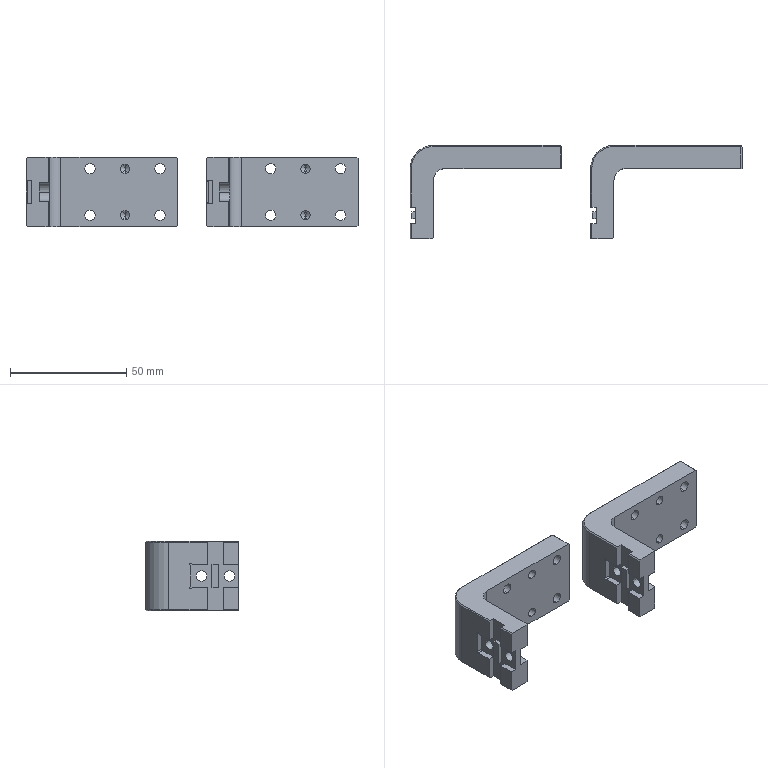NC program | NX | posted with a generic post | part box 142.5 x 40 x 30 mm
Whole program:
N10 G17 G21 G94 G90
(FLOOR_WALL_1 , TOOL : D2)
N12 T17 M6
N14 G54
N16 G17 G0 G90 X1.559 Y-22.5 B0. C0. S9500 M3
N18 G43 Z30. H17
N20 Z0.853
N22 G94 G1 Z-0.147 F1250.
N24 X0.173 Y-20.1
N26 G3 X0. Y-20. R0.2
N28 G1 X-4.
N30 Y-12.75
N32 X4.
N34 Y-20.
N36 X0.
N38 Y-19.
N40 X-3.
N42 Y-13.75
N44 X3.
N46 Y-19.
N48 X0.
N50 Y-18.
N52 X-2.
N54 Y-14.75
N56 X2.
N58 Y-18.
N60 X0.
N62 Y-17.
N64 X-1.
N66 Y-15.75
N68 X1.
N70 Y-17.
N72 X0.
N74 G3 X-0.173 Y-17.1 R0.2
N76 G1 Y-22.5
N78 Z0.853
N80 G0 Z30.
N82 X2.453 Y-0.55
N84 Z0.5
N86 G1 X4. Z0.419
N88 Y-7.35 Z0.063
N90 X0. Z-0.147
N92 X-4.
N94 Y-0.55
N96 X4.
N98 Y-7.35
N100 X0.
N102 Y-6.35
N104 X-3.
N106 Y-1.55
N108 X3.
N110 Y-6.35
N112 X0.
N114 Y-5.35
N116 X-2.
N118 Y-2.55
N120 X2.
N122 Y-5.35
N124 X0.
N126 Y-4.35
N128 X-1.
N130 Y-3.55
N132 X1.
N134 Y-4.35
N136 X0.
N138 G3 X-0.173 Y-4.45 R0.2
N140 G1 Z0.853
N142 G0 Z30.
N144 X-17.5 Y-11.609
N146 Z0.853
N148 G1 Z-0.147
N150 X-15.1 Y-10.223
N152 G3 X-15. Y-10.05 R0.2
N154 G1 Y-7.55
N156 X-6.2
N158 Y-12.55
N160 X-15.
N162 Y-10.05
N164 X-14.
N166 Y-8.55
N168 X-7.2
N170 Y-11.55
N172 X-14.
N174 Y-10.05
N176 X-13.
N178 Y-9.55
N180 X-8.2
N182 Y-10.55
N184 X-13.
N186 Y-10.05
N188 G3 X-13.1 Y-9.877 R0.2
N190 G1 X-17.5
N192 Z0.853
N194 G0 Z30.
N196 X17.5 Y-8.491
N198 Z0.853
N200 G1 Z-0.147
N202 X15.1 Y-9.877
N204 G3 X15. Y-10.05 R0.2
N206 G1 Y-12.55
N208 X6.2
N210 Y-7.55
N212 X6.
N214 Y-12.55
N216 X-6.
N218 Y-7.55
N220 X6.
N222 X6.2
N224 X15.
N226 Y-10.05
N228 X14.
N230 Y-11.55
N232 X7.2
N234 Y-8.55
N236 X14.
N238 Y-10.05
N240 X13.
N242 Y-10.55
N244 X8.2
N246 Y-9.55
N248 X13.
N250 Y-10.05
N252 G3 X13.1 Y-10.223 R0.2
N254 G1 X17.5
N256 Z0.853
N258 G0 Z30.
N260 X1.559 Y-22.5
N262 Z0.706
N264 G1 Z-0.294
N266 X0.173 Y-20.1
N268 G3 X0. Y-20. R0.2
N270 G1 X-4.
N272 Y-12.75
N274 X4.
N276 Y-20.
N278 X0.
N280 Y-19.
N282 X-3.
N284 Y-13.75
N286 X3.
N288 Y-19.
N290 X0.
N292 Y-18.
N294 X-2.
N296 Y-14.75
N298 X2.
N300 Y-18.
N302 X0.
N304 Y-17.
N306 X-1.
N308 Y-15.75
N310 X1.
N312 Y-17.
N314 X0.
N316 G3 X-0.173 Y-17.1 R0.2
N318 G1 Y-22.5
N320 Z0.706
N322 G0 Z30.
N324 X2.453 Y-0.55
N326 Z0.353
N328 G1 X4. Z0.272
N330 Y-7.35 Z-0.084
N332 X0. Z-0.294
N334 X-4.
N336 Y-0.55
N338 X4.
N340 Y-7.35
N342 X0.
N344 Y-6.35
N346 X-3.
N348 Y-1.55
N350 X3.
N352 Y-6.35
N354 X0.
N356 Y-5.35
N358 X-2.
N360 Y-2.55
N362 X2.
N364 Y-5.35
N366 X0.
N368 Y-4.35
N370 X-1.
N372 Y-3.55
N374 X1.
N376 Y-4.35
N378 X0.
N380 G3 X-0.173 Y-4.45 R0.2
N382 G1 Z0.706
N384 G0 Z30.
N386 X17.5 Y-8.491
N388 Z0.706
N390 G1 Z-0.294
N392 X15.1 Y-9.877
N394 G3 X15. Y-10.05 R0.2
N396 G1 Y-12.55
N398 X6.2
N400 Y-7.55
N402 X15.
N404 Y-10.05
N406 X14.
N408 Y-11.55
N410 X7.2
N412 Y-8.55
N414 X14.
N416 Y-10.05
N418 X13.
N420 Y-10.55
N422 X8.2
N424 Y-9.55
N426 X13.
N428 Y-10.05
N430 G3 X13.1 Y-10.223 R0.2
N432 G1 X17.5
N434 Z0.706
N436 G0 Z30.
N438 X-17.5 Y-11.609
N440 Z0.706
N442 G1 Z-0.294
N444 X-15.1 Y-10.223
N446 G3 X-15. Y-10.05 R0.2
N448 G1 Y-7.55
N450 X-6.2
N452 Y-12.55
N454 X-6.
N456 Y-7.55
N458 X6.
N460 Y-12.55
N462 X-6.
N464 X-6.2
N466 X-15.
N468 Y-10.05
N470 X-14.
N472 Y-8.55
N474 X-7.2
N476 Y-11.55
N478 X-14.
N480 Y-10.05
N482 X-13.
N484 Y-9.55
N486 X-8.2
N488 Y-10.55
N490 X-13.
N492 Y-10.05
N494 G3 X-13.1 Y-9.877 R0.2
N496 G1 X-17.5
N498 Z0.706
N500 G0 Z30.
N502 X1.559 Y-22.5
N504 Z0.559
N506 G1 Z-0.441
N508 X0.173 Y-20.1
N510 G3 X0. Y-20. R0.2
N512 G1 X-4.
N514 Y-12.75
N516 X4.
N518 Y-20.
N520 X0.
N522 Y-19.
N524 X-3.
N526 Y-13.75
N528 X3.
N530 Y-19.
N532 X0.
N534 Y-18.
N536 X-2.
N538 Y-14.75
N540 X2.
N542 Y-18.
N544 X0.
N546 Y-17.
N548 X-1.
N550 Y-15.75
N552 X1.
N554 Y-17.
N556 X0.
N558 G3 X-0.173 Y-17.1 R0.2
N560 G1 Y-22.5
N562 Z0.559
N564 G0 Z30.
N566 X2.453 Y-0.55
N568 Z0.206
N570 G1 X4. Z0.125
N572 Y-7.35 Z-0.232
N574 X0. Z-0.441
N576 X-4.
N578 Y-0.55
N580 X4.
N582 Y-7.35
N584 X0.
N586 Y-6.35
N588 X-3.
N590 Y-1.55
N592 X3.
N594 Y-6.35
N596 X0.
N598 Y-5.35
N600 X-2.
N602 Y-2.55
N604 X2.
N606 Y-5.35
N608 X0.
N610 Y-4.35
N612 X-1.
N614 Y-3.55
N616 X1.
N618 Y-4.35
N620 X0.
N622 G3 X-0.173 Y-4.45 R0.2
N624 G1 Z0.559
N626 G0 Z30.
N628 X-17.5 Y-11.609
N630 Z0.559
N632 G1 Z-0.441
N634 X-15.1 Y-10.223
N636 G3 X-15. Y-10.05 R0.2
N638 G1 Y-7.55
N640 X-6.2
N642 Y-12.55
N644 X-15.
N646 Y-10.05
N648 X-14.
N650 Y-8.55
N652 X-7.2
N654 Y-11.55
N656 X-14.
N658 Y-10.05
N660 X-13.
N662 Y-9.55
N664 X-8.2
N666 Y-10.55
N668 X-13.
N670 Y-10.05
N672 G3 X-13.1 Y-9.877 R0.2
N674 G1 X-17.5
N676 Z0.559
N678 G0 Z30.
N680 X17.5 Y-8.491
N682 Z0.559
N684 G1 Z-0.441
N686 X15.1 Y-9.877
N688 G3 X15. Y-10.05 R0.2
N690 G1 Y-12.55
N692 X6.2
N694 Y-7.55
N696 X6.
N698 Y-12.55
N700 X-6.
N702 Y-7.55
N704 X6.
N706 X6.2
N708 X15.
N710 Y-10.05
N712 X14.
N714 Y-11.55
N716 X7.2
N718 Y-8.55
N720 X14.
N722 Y-10.05
N724 X13.
N726 Y-10.55
N728 X8.2
N730 Y-9.55
N732 X13.
N734 Y-10.05
N736 G3 X13.1 Y-10.223 R0.2
N738 G1 X17.5
N740 Z0.559
N742 G0 Z30.
N744 X1.559 Y-22.5
N746 Z0.412
N748 G1 Z-0.588
N750 X0.173 Y-20.1
N752 G3 X0. Y-20. R0.2
N754 G1 X-4.
N756 Y-12.75
N758 X4.
N760 Y-20.
N762 X0.
N764 Y-19.
N766 X-3.
N768 Y-13.75
N770 X3.
N772 Y-19.
N774 X0.
N776 Y-18.
N778 X-2.
N780 Y-14.75
N782 X2.
N784 Y-18.
N786 X0.
N788 Y-17.
N790 X-1.
N792 Y-15.75
N794 X1.
N796 Y-17.
N798 X0.
N800 G3 X-0.173 Y-17.1 R0.2
N802 G1 Y-22.5
N804 Z0.412
N806 G0 Z30.
N808 X2.453 Y-0.55
N810 Z0.059
N812 G1 X4. Z-0.022
N814 Y-7.35 Z-0.379
N816 X0. Z-0.588
N818 X-4.
N820 Y-0.55
N822 X4.
N824 Y-7.35
N826 X0.
N828 Y-6.35
N830 X-3.
N832 Y-1.55
N834 X3.
N836 Y-6.35
N838 X0.
N840 Y-5.35
N842 X-2.
N844 Y-2.55
N846 X2.
N848 Y-5.35
N850 X0.
N852 Y-4.35
N854 X-1.
N856 Y-3.55
N858 X1.
N860 Y-4.35
N862 X0.
N864 G3 X-0.173 Y-4.45 R0.2
N866 G1 Z0.412
N868 G0 Z30.
N870 X17.5 Y-8.491
N872 Z0.412
N874 G1 Z-0.588
N876 X15.1 Y-9.877
N878 G3 X15. Y-10.05 R0.2
N880 G1 Y-12.55
N882 X6.2
N884 Y-7.55
N886 X15.
N888 Y-10.05
N890 X14.
N892 Y-11.55
N894 X7.2
N896 Y-8.55
N898 X14.
N900 Y-10.05
N902 X13.
N904 Y-10.55
N906 X8.2
N908 Y-9.55
N910 X13.
N912 Y-10.05
N914 G3 X13.1 Y-10.223 R0.2
N916 G1 X17.5
N918 Z0.412
N920 G0 Z30.
N922 X-17.5 Y-11.609
N924 Z0.412
N926 G1 Z-0.588
N928 X-15.1 Y-10.223
N930 G3 X-15. Y-10.05 R0.2
N932 G1 Y-7.55
N934 X-6.2
N936 Y-12.55
N938 X-6.
N940 Y-7.55
N942 X6.
N944 Y-12.55
N946 X-6.
N948 X-6.2
N950 X-15.
N952 Y-10.05
N954 X-14.
N956 Y-8.55
N958 X-7.2
N960 Y-11.55
N962 X-14.
N964 Y-10.05
N966 X-13.
N968 Y-9.55
N970 X-8.2
N972 Y-10.55
N974 X-13.
N976 Y-10.05
N978 G3 X-13.1 Y-9.877 R0.2
N980 G1 X-17.5
N982 Z0.412
N984 G0 Z30.
N986 X1.559 Y-22.5
N988 Z0.265
N990 G1 Z-0.735
N992 X0.173 Y-20.1
N994 G3 X0. Y-20. R0.2
N996 G1 X-4.
N998 Y-12.75
N1000 X4.
N1002 Y-20.
N1004 X0.
N1006 Y-19.
N1008 X-3.
N1010 Y-13.75
N1012 X3.
N1014 Y-19.
N1016 X0.
N1018 Y-18.
N1020 X-2.
N1022 Y-14.75
N1024 X2.
N1026 Y-18.
N1028 X0.
N1030 Y-17.
N1032 X-1.
N1034 Y-15.75
N1036 X1.
N1038 Y-17.
N1040 X0.
N1042 G3 X-0.173 Y-17.1 R0.2
N1044 G1 Y-22.5
N1046 Z0.265
N1048 G0 Z30.
N1050 X2.453 Y-0.55
N1052 Z-0.088
N1054 G1 X4. Z-0.169
N1056 Y-7.35 Z-0.526
N1058 X0. Z-0.735
N1060 X-4.
N1062 Y-0.55
N1064 X4.
N1066 Y-7.35
N1068 X0.
N1070 Y-6.35
N1072 X-3.
N1074 Y-1.55
N1076 X3.
N1078 Y-6.35
N1080 X0.
N1082 Y-5.35
N1084 X-2.
N1086 Y-2.55
N1088 X2.
N1090 Y-5.35
N1092 X0.
N1094 Y-4.35
N1096 X-1.
N1098 Y-3.55
N1100 X1.
N1102 Y-4.35
N1104 X0.
N1106 G3 X-0.173 Y-4.45 R0.2
N1108 G1 Z0.265
N1110 G0 Z30.
N1112 X-17.5 Y-11.609
N1114 Z0.265
N1116 G1 Z-0.735
N1118 X-15.1 Y-10.223
N1120 G3 X-15. Y-10.05 R0.2
N1122 G1 Y-7.55
N1124 X-6.2
N1126 Y-12.55
N1128 X-15.
N1130 Y-10.05
N1132 X-14.
N1134 Y-8.55
N1136 X-7.2
N1138 Y-11.55
N1140 X-14.
N1142 Y-10.05
N1144 X-13.
N1146 Y-9.55
N1148 X-8.2
N1150 Y-10.55
N1152 X-13.
N1154 Y-10.05
N1156 G3 X-13.1 Y-9.877 R0.2
N1158 G1 X-17.5
N1160 Z0.265
N1162 G0 Z30.
N1164 X17.5 Y-8.491
N1166 Z0.265
N1168 G1 Z-0.735
N1170 X15.1 Y-9.877
N1172 G3 X15. Y-10.05 R0.2
N1174 G1 Y-12.55
N1176 X6.2
N1178 Y-7.55
N1180 X6.
N1182 Y-12.55
N1184 X-6.
N1186 Y-7.55
N1188 X6.
N1190 X6.2
N1192 X15.
N1194 Y-10.05
N1196 X14.
N1198 Y-11.55
N1200 X7.2
N1202 Y-8.55
N1204 X14.
N1206 Y-10.05
N1208 X13.
N1210 Y-10.55
N1212 X8.2
N1214 Y-9.55
N1216 X13.
N1218 Y-10.05
N1220 G3 X13.1 Y-10.223 R0.2
N1222 G1 X17.5
N1224 Z0.265
N1226 G0 Z30.
N1228 X1.559 Y-22.5
N1230 Z0.118
N1232 G1 Z-0.882
N1234 X0.173 Y-20.1
N1236 G3 X0. Y-20. R0.2
N1238 G1 X-4.
N1240 Y-12.75
N1242 X4.
N1244 Y-20.
N1246 X0.
N1248 Y-19.
N1250 X-3.
N1252 Y-13.75
N1254 X3.
N1256 Y-19.
N1258 X0.
N1260 Y-18.
N1262 X-2.
N1264 Y-14.75
N1266 X2.
N1268 Y-18.
N1270 X0.
N1272 Y-17.
N1274 X-1.
N1276 Y-15.75
N1278 X1.
N1280 Y-17.
N1282 X0.
N1284 G3 X-0.173 Y-17.1 R0.2
N1286 G1 Y-22.5
N1288 Z0.118
N1290 G0 Z30.
N1292 X2.453 Y-0.55
N1294 Z-0.235
N1296 G1 X4. Z-0.316
N1298 Y-7.35 Z-0.673
N1300 X0. Z-0.882
N1302 X-4.
N1304 Y-0.55
N1306 X4.
N1308 Y-7.35
N1310 X0.
N1312 Y-6.35
N1314 X-3.
N1316 Y-1.55
N1318 X3.
N1320 Y-6.35
N1322 X0.
N1324 Y-5.35
N1326 X-2.
N1328 Y-2.55
N1330 X2.
N1332 Y-5.35
N1334 X0.
N1336 Y-4.35
N1338 X-1.
N1340 Y-3.55
N1342 X1.
N1344 Y-4.35
N1346 X0.
N1348 G3 X-0.173 Y-4.45 R0.2
N1350 G1 Z0.118
N1352 G0 Z30.
N1354 X17.5 Y-8.491
N1356 Z0.118
N1358 G1 Z-0.882
N1360 X15.1 Y-9.877
N1362 G3 X15. Y-10.05 R0.2
N1364 G1 Y-12.55
N1366 X6.2
N1368 Y-7.55
N1370 X15.
N1372 Y-10.05
N1374 X14.
N1376 Y-11.55
N1378 X7.2
N1380 Y-8.55
N1382 X14.
N1384 Y-10.05
N1386 X13.
N1388 Y-10.55
N1390 X8.2
N1392 Y-9.55
N1394 X13.
N1396 Y-10.05
N1398 G3 X13.1 Y-10.223 R0.2
N1400 G1 X17.5
N1402 Z0.118
N1404 G0 Z30.
N1406 X-17.5 Y-11.609
N1408 Z0.118
N1410 G1 Z-0.882
N1412 X-15.1 Y-10.223
N1414 G3 X-15. Y-10.05 R0.2
N1416 G1 Y-7.55
N1418 X-6.2
N1420 Y-12.55
N1422 X-6.
N1424 Y-7.55
N1426 X6.
N1428 Y-12.55
N1430 X-6.
N1432 X-6.2
N1434 X-15.
N1436 Y-10.05
N1438 X-14.
N1440 Y-8.55
N1442 X-7.2
N1444 Y-11.55
N1446 X-14.
N1448 Y-10.05
N1450 X-13.
N1452 Y-9.55
N1454 X-8.2
N1456 Y-10.55
N1458 X-13.
N1460 Y-10.05
N1462 G3 X-13.1 Y-9.877 R0.2
N1464 G1 X-17.5
N1466 Z0.118
N1468 G0 Z30.
N1470 X1.559 Y-22.5
N1472 Z-0.029
N1474 G1 Z-1.029
N1476 X0.173 Y-20.1
N1478 G3 X0. Y-20. R0.2
N1480 G1 X-4.
N1482 Y-12.75
N1484 X4.
N1486 Y-20.
N1488 X0.
N1490 Y-19.
N1492 X-3.
N1494 Y-13.75
N1496 X3.
N1498 Y-19.
N1500 X0.
N1502 Y-18.
N1504 X-2.
N1506 Y-14.75
N1508 X2.
N1510 Y-18.
N1512 X0.
N1514 Y-17.
N1516 X-1.
N1518 Y-15.75
N1520 X1.
N1522 Y-17.
N1524 X0.
N1526 G3 X-0.173 Y-17.1 R0.2
N1528 G1 Y-22.5
N1530 Z-0.029
N1532 G0 Z30.
N1534 X2.453 Y-0.55
N1536 Z-0.382
N1538 G1 X4. Z-0.463
N1540 Y-7.35 Z-0.82
N1542 X0. Z-1.029
N1544 X-4.
N1546 Y-0.55
N1548 X4.
N1550 Y-7.35
N1552 X0.
N1554 Y-6.35
N1556 X-3.
N1558 Y-1.55
N1560 X3.
N1562 Y-6.35
N1564 X0.
N1566 Y-5.35
N1568 X-2.
N1570 Y-2.55
N1572 X2.
N1574 Y-5.35
N1576 X0.
N1578 Y-4.35
N1580 X-1.
N1582 Y-3.55
N1584 X1.
N1586 Y-4.35
N1588 X0.
N1590 G3 X-0.173 Y-4.45 R0.2
N1592 G1 Z-0.029
N1594 G0 Z30.
N1596 X-17.5 Y-11.609
N1598 Z-0.029
N1600 G1 Z-1.029
N1602 X-15.1 Y-10.223
N1604 G3 X-15. Y-10.05 R0.2
N1606 G1 Y-7.55
N1608 X-6.2
N1610 Y-12.55
N1612 X-15.
N1614 Y-10.05
N1616 X-14.
N1618 Y-8.55
N1620 X-7.2
N1622 Y-11.55
N1624 X-14.
N1626 Y-10.05
N1628 X-13.
N1630 Y-9.55
N1632 X-8.2
N1634 Y-10.55
N1636 X-13.
N1638 Y-10.05
N1640 G3 X-13.1 Y-9.877 R0.2
N1642 G1 X-17.5
N1644 Z-0.029
N1646 G0 Z30.
N1648 X17.5 Y-8.491
N1650 Z-0.029
N1652 G1 Z-1.029
N1654 X15.1 Y-9.877
N1656 G3 X15. Y-10.05 R0.2
N1658 G1 Y-12.55
N1660 X6.2
N1662 Y-7.55
N1664 X6.
N1666 Y-12.55
N1668 X-6.
N1670 Y-7.55
N1672 X6.
N1674 X6.2
N1676 X15.
N1678 Y-10.05
N1680 X14.
N1682 Y-11.55
N1684 X7.2
N1686 Y-8.55
N1688 X14.
N1690 Y-10.05
N1692 X13.
N1694 Y-10.55
N1696 X8.2
N1698 Y-9.55
N1700 X13.
N1702 Y-10.05
N1704 G3 X13.1 Y-10.223 R0.2
N1706 G1 X17.5
N1708 Z-0.029
N1710 G0 Z30.
N1712 X1.559 Y-22.5
N1714 Z-0.176
N1716 G1 Z-1.176
N1718 X0.173 Y-20.1
N1720 G3 X0. Y-20. R0.2
N1722 G1 X-4.
N1724 Y-12.75
N1726 X4.
N1728 Y-20.
N1730 X0.
N1732 Y-19.
N1734 X-3.
N1736 Y-13.75
N1738 X3.
N1740 Y-19.
N1742 X0.
N1744 Y-18.
N1746 X-2.
N1748 Y-14.75
N1750 X2.
N1752 Y-18.
N1754 X0.
N1756 Y-17.
N1758 X-1.
N1760 Y-15.75
N1762 X1.
N1764 Y-17.
N1766 X0.
N1768 G3 X-0.173 Y-17.1 R0.2
N1770 G1 Y-22.5
N1772 Z-0.176
N1774 G0 Z30.
N1776 X2.453 Y-0.55
N1778 Z-0.529
N1780 G1 X4. Z-0.61
N1782 Y-7.35 Z-0.967
N1784 X0. Z-1.176
N1786 X-4.
N1788 Y-0.55
N1790 X4.
N1792 Y-7.35
N1794 X0.
N1796 Y-6.35
N1798 X-3.
N1800 Y-1.55
N1802 X3.
N1804 Y-6.35
N1806 X0.
N1808 Y-5.35
N1810 X-2.
N1812 Y-2.55
N1814 X2.
N1816 Y-5.35
N1818 X0.
N1820 Y-4.35
N1822 X-1.
N1824 Y-3.55
N1826 X1.
N1828 Y-4.35
N1830 X0.
N1832 G3 X-0.173 Y-4.45 R0.2
N1834 G1 Z-0.176
N1836 G0 Z30.
N1838 X17.5 Y-8.491
N1840 Z-0.176
N1842 G1 Z-1.176
N1844 X15.1 Y-9.877
N1846 G3 X15. Y-10.05 R0.2
N1848 G1 Y-12.55
N1850 X6.2
N1852 Y-7.55
N1854 X15.
N1856 Y-10.05
N1858 X14.
N1860 Y-11.55
N1862 X7.2
N1864 Y-8.55
N1866 X14.
N1868 Y-10.05
N1870 X13.
N1872 Y-10.55
N1874 X8.2
N1876 Y-9.55
N1878 X13.
N1880 Y-10.05
N1882 G3 X13.1 Y-10.223 R0.2
N1884 G1 X17.5
N1886 Z-0.176
N1888 G0 Z30.
N1890 X-17.5 Y-11.609
N1892 Z-0.176
N1894 G1 Z-1.176
N1896 X-15.1 Y-10.223
N1898 G3 X-15. Y-10.05 R0.2
N1900 G1 Y-7.55
N1902 X-6.2
N1904 Y-12.55
N1906 X-6.
N1908 Y-7.55
N1910 X6.
N1912 Y-12.55
N1914 X-6.
N1916 X-6.2
N1918 X-15.
N1920 Y-10.05
N1922 X-14.
N1924 Y-8.55
N1926 X-7.2
N1928 Y-11.55
N1930 X-14.
N1932 Y-10.05
N1934 X-13.
N1936 Y-9.55
N1938 X-8.2
N1940 Y-10.55
N1942 X-13.
N1944 Y-10.05
N1946 G3 X-13.1 Y-9.877 R0.2
N1948 G1 X-17.5
N1950 Z-0.176
N1952 G0 Z30.
N1954 X1.559 Y-22.5
N1956 Z-0.324
N1958 G1 Z-1.324
N1960 X0.173 Y-20.1
N1962 G3 X0. Y-20. R0.2
N1964 G1 X-4.
N1966 Y-12.75
N1968 X4.
N1970 Y-20.
N1972 X0.
N1974 Y-19.
N1976 X-3.
N1978 Y-13.75
N1980 X3.
N1982 Y-19.
N1984 X0.
N1986 Y-18.
N1988 X-2.
N1990 Y-14.75
N1992 X2.
N1994 Y-18.
N1996 X0.
N1998 Y-17.
N2000 X-1.
N2002 Y-15.75
N2004 X1.
N2006 Y-17.
N2008 X0.
N2010 G3 X-0.173 Y-17.1 R0.2
N2012 G1 Y-22.5
N2014 Z-0.324
N2016 G0 Z30.
N2018 X2.453 Y-0.55
N2020 Z-0.676
N2022 G1 X4. Z-0.758
N2024 Y-7.35 Z-1.114
N2026 X0. Z-1.324
N2028 X-4.
N2030 Y-0.55
N2032 X4.
N2034 Y-7.35
N2036 X0.
N2038 Y-6.35
N2040 X-3.
N2042 Y-1.55
N2044 X3.
N2046 Y-6.35
N2048 X0.
N2050 Y-5.35
N2052 X-2.
N2054 Y-2.55
N2056 X2.
N2058 Y-5.35
N2060 X0.
N2062 Y-4.35
N2064 X-1.
N2066 Y-3.55
N2068 X1.
N2070 Y-4.35
N2072 X0.
N2074 G3 X-0.173 Y-4.45 R0.2
N2076 G1 Z-0.324
N2078 G0 Z30.
N2080 X-17.5 Y-11.609
N2082 Z-0.324
N2084 G1 Z-1.324
N2086 X-15.1 Y-10.223
N2088 G3 X-15. Y-10.05 R0.2
N2090 G1 Y-7.55
N2092 X-6.2
N2094 Y-12.55
N2096 X-15.
N2098 Y-10.05
N2100 X-14.
N2102 Y-8.55
N2104 X-7.2
N2106 Y-11.55
N2108 X-14.
N2110 Y-10.05
N2112 X-13.
N2114 Y-9.55
N2116 X-8.2
N2118 Y-10.55
N2120 X-13.
N2122 Y-10.05
N2124 G3 X-13.1 Y-9.877 R0.2
N2126 G1 X-17.5
N2128 Z-0.324
N2130 G0 Z30.
N2132 X17.5 Y-8.491
N2134 Z-0.324
N2136 G1 Z-1.324
N2138 X15.1 Y-9.877
N2140 G3 X15. Y-10.05 R0.2
N2142 G1 Y-12.55
N2144 X6.2
N2146 Y-7.55
N2148 X6.
N2150 Y-12.55
N2152 X-6.
N2154 Y-7.55
N2156 X6.
N2158 X6.2
N2160 X15.
N2162 Y-10.05
N2164 X14.
N2166 Y-11.55
N2168 X7.2
N2170 Y-8.55
N2172 X14.
N2174 Y-10.05
N2176 X13.
N2178 Y-10.55
N2180 X8.2
N2182 Y-9.55
N2184 X13.
N2186 Y-10.05
N2188 G3 X13.1 Y-10.223 R0.2
N2190 G1 X17.5
N2192 Z-0.324
N2194 G0 Z30.
N2196 X1.559 Y-22.5
N2198 Z-0.471
N2200 G1 Z-1.471
N2202 X0.173 Y-20.1
N2204 G3 X0. Y-20. R0.2
N2206 G1 X-4.
N2208 Y-12.75
N2210 X4.
N2212 Y-20.
N2214 X0.
N2216 Y-19.
N2218 X-3.
N2220 Y-13.75
N2222 X3.
N2224 Y-19.
N2226 X0.
N2228 Y-18.
N2230 X-2.
N2232 Y-14.75
N2234 X2.
N2236 Y-18.
N2238 X0.
N2240 Y-17.
N2242 X-1.
N2244 Y-15.75
N2246 X1.
N2248 Y-17.
N2250 X0.
N2252 G3 X-0.173 Y-17.1 R0.2
N2254 G1 Y-22.5
N2256 Z-0.471
N2258 G0 Z30.
N2260 X2.453 Y-0.55
N2262 Z-0.824
N2264 G1 X4. Z-0.905
N2266 Y-7.35 Z-1.261
N2268 X0. Z-1.471
N2270 X-4.
N2272 Y-0.55
N2274 X4.
N2276 Y-7.35
N2278 X0.
N2280 Y-6.35
N2282 X-3.
N2284 Y-1.55
N2286 X3.
N2288 Y-6.35
N2290 X0.
N2292 Y-5.35
N2294 X-2.
N2296 Y-2.55
N2298 X2.
N2300 Y-5.35
N2302 X0.
N2304 Y-4.35
N2306 X-1.
N2308 Y-3.55
N2310 X1.
N2312 Y-4.35
N2314 X0.
N2316 G3 X-0.173 Y-4.45 R0.2
N2318 G1 Z-0.471
N2320 G0 Z30.
N2322 X17.5 Y-8.491
N2324 Z-0.471
N2326 G1 Z-1.471
N2328 X15.1 Y-9.877
N2330 G3 X15. Y-10.05 R0.2
N2332 G1 Y-12.55
N2334 X6.2
N2336 Y-7.55
N2338 X15.
N2340 Y-10.05
N2342 X14.
N2344 Y-11.55
N2346 X7.2
N2348 Y-8.55
N2350 X14.
N2352 Y-10.05
N2354 X13.
N2356 Y-10.55
N2358 X8.2
N2360 Y-9.55
N2362 X13.
N2364 Y-10.05
N2366 G3 X13.1 Y-10.223 R0.2
N2368 G1 X17.5
N2370 Z-0.471
N2372 G0 Z30.
N2374 X-17.5 Y-11.609
N2376 Z-0.471
N2378 G1 Z-1.471
N2380 X-15.1 Y-10.223
N2382 G3 X-15. Y-10.05 R0.2
N2384 G1 Y-7.55
N2386 X-6.2
N2388 Y-12.55
N2390 X-6.
N2392 Y-7.55
N2394 X6.
N2396 Y-12.55
N2398 X-6.
N2400 X-6.2
N2402 X-15.
N2404 Y-10.05
N2406 X-14.
N2408 Y-8.55
N2410 X-7.2
N2412 Y-11.55
N2414 X-14.
N2416 Y-10.05
N2418 X-13.
N2420 Y-9.55
N2422 X-8.2
N2424 Y-10.55
N2426 X-13.
N2428 Y-10.05
N2430 G3 X-13.1 Y-9.877 R0.2
N2432 G1 X-17.5
N2434 Z-0.471
N2436 G0 Z30.
N2438 X1.559 Y-22.5
N2440 Z-0.618
N2442 G1 Z-1.618
N2444 X0.173 Y-20.1
N2446 G3 X0. Y-20. R0.2
N2448 G1 X-4.
N2450 Y-12.75
N2452 X4.
N2454 Y-20.
N2456 X0.
N2458 Y-19.
N2460 X-3.
N2462 Y-13.75
N2464 X3.
N2466 Y-19.
N2468 X0.
N2470 Y-18.
N2472 X-2.
N2474 Y-14.75
N2476 X2.
N2478 Y-18.
N2480 X0.
N2482 Y-17.
N2484 X-1.
N2486 Y-15.75
N2488 X1.
N2490 Y-17.
N2492 X0.
N2494 G3 X-0.173 Y-17.1 R0.2
N2496 G1 Y-22.5
N2498 Z-0.618
N2500 G0 Z30.
N2502 X2.453 Y-0.55
N2504 Z-0.971
N2506 G1 X4. Z-1.052
N2508 Y-7.35 Z-1.408
N2510 X0. Z-1.618
N2512 X-4.
N2514 Y-0.55
N2516 X4.
N2518 Y-7.35
N2520 X0.
N2522 Y-6.35
N2524 X-3.
N2526 Y-1.55
N2528 X3.
N2530 Y-6.35
N2532 X0.
N2534 Y-5.35
N2536 X-2.
N2538 Y-2.55
N2540 X2.
N2542 Y-5.35
N2544 X0.
N2546 Y-4.35
N2548 X-1.
N2550 Y-3.55
N2552 X1.
N2554 Y-4.35
N2556 X0.
N2558 G3 X-0.173 Y-4.45 R0.2
N2560 G1 Z-0.618
N2562 G0 Z30.
N2564 X-17.5 Y-11.609
N2566 Z-0.618
N2568 G1 Z-1.618
N2570 X-15.1 Y-10.223
N2572 G3 X-15. Y-10.05 R0.2
N2574 G1 Y-7.55
N2576 X-6.2
N2578 Y-12.55
N2580 X-15.
N2582 Y-10.05
N2584 X-14.
N2586 Y-8.55
N2588 X-7.2
N2590 Y-11.55
N2592 X-14.
N2594 Y-10.05
N2596 X-13.
N2598 Y-9.55
N2600 X-8.2
N2602 Y-10.55
N2604 X-13.
N2606 Y-10.05
N2608 G3 X-13.1 Y-9.877 R0.2
N2610 G1 X-17.5
N2612 Z-0.618
N2614 G0 Z30.
N2616 X17.5 Y-8.491
N2618 Z-0.618
N2620 G1 Z-1.618
N2622 X15.1 Y-9.877
N2624 G3 X15. Y-10.05 R0.2
N2626 G1 Y-12.55
N2628 X6.2
N2630 Y-7.55
N2632 X6.
N2634 Y-12.55
N2636 X-6.
N2638 Y-7.55
N2640 X6.
N2642 X6.2
N2644 X15.
N2646 Y-10.05
N2648 X14.
N2650 Y-11.55
N2652 X7.2
N2654 Y-8.55
N2656 X14.
N2658 Y-10.05
N2660 X13.
N2662 Y-10.55
N2664 X8.2
N2666 Y-9.55
N2668 X13.
N2670 Y-10.05
N2672 G3 X13.1 Y-10.223 R0.2
N2674 G1 X17.5
N2676 Z-0.618
N2678 G0 Z30.
N2680 X1.559 Y-22.5
N2682 Z-0.765
N2684 G1 Z-1.765
N2686 X0.173 Y-20.1
N2688 G3 X0. Y-20. R0.2
N2690 G1 X-4.
N2692 Y-12.75
N2694 X4.
N2696 Y-20.
N2698 X0.
N2700 Y-19.
N2702 X-3.
N2704 Y-13.75
N2706 X3.
N2708 Y-19.
N2710 X0.
N2712 Y-18.
N2714 X-2.
N2716 Y-14.75
N2718 X2.
N2720 Y-18.
N2722 X0.
N2724 Y-17.
N2726 X-1.
N2728 Y-15.75
N2730 X1.
N2732 Y-17.
N2734 X0.
N2736 G3 X-0.173 Y-17.1 R0.2
N2738 G1 Y-22.5
N2740 Z-0.765
N2742 G0 Z30.
N2744 X2.453 Y-0.55
N2746 Z-1.118
N2748 G1 X4. Z-1.199
N2750 Y-7.35 Z-1.555
N2752 X0. Z-1.765
N2754 X-4.
N2756 Y-0.55
N2758 X4.
N2760 Y-7.35
N2762 X0.
N2764 Y-6.35
N2766 X-3.
N2768 Y-1.55
N2770 X3.
N2772 Y-6.35
N2774 X0.
N2776 Y-5.35
N2778 X-2.
N2780 Y-2.55
N2782 X2.
N2784 Y-5.35
N2786 X0.
N2788 Y-4.35
N2790 X-1.
N2792 Y-3.55
N2794 X1.
N2796 Y-4.35
N2798 X0.
N2800 G3 X-0.173 Y-4.45 R0.2
N2802 G1 Z-0.765
N2804 G0 Z30.
N2806 X17.5 Y-8.491
N2808 Z-0.765
N2810 G1 Z-1.765
N2812 X15.1 Y-9.877
N2814 G3 X15. Y-10.05 R0.2
N2816 G1 Y-12.55
N2818 X6.2
N2820 Y-7.55
N2822 X15.
N2824 Y-10.05
N2826 X14.
N2828 Y-11.55
N2830 X7.2
N2832 Y-8.55
N2834 X14.
N2836 Y-10.05
N2838 X13.
N2840 Y-10.55
N2842 X8.2
N2844 Y-9.55
N2846 X13.
N2848 Y-10.05
N2850 G3 X13.1 Y-10.223 R0.2
N2852 G1 X17.5
N2854 Z-0.765
N2856 G0 Z30.
N2858 X-17.5 Y-11.609
N2860 Z-0.765
N2862 G1 Z-1.765
N2864 X-15.1 Y-10.223
N2866 G3 X-15. Y-10.05 R0.2
N2868 G1 Y-7.55
N2870 X-6.2
N2872 Y-12.55
N2874 X-6.
N2876 Y-7.55
N2878 X6.
N2880 Y-12.55
N2882 X-6.
N2884 X-6.2
N2886 X-15.
N2888 Y-10.05
N2890 X-14.
N2892 Y-8.55
N2894 X-7.2
N2896 Y-11.55
N2898 X-14.
N2900 Y-10.05
N2902 X-13.
N2904 Y-9.55
N2906 X-8.2
N2908 Y-10.55
N2910 X-13.
N2912 Y-10.05
N2914 G3 X-13.1 Y-9.877 R0.2
N2916 G1 X-17.5
N2918 Z-0.765
N2920 G0 Z30.
N2922 X1.559 Y-22.5
N2924 Z-0.912
N2926 G1 Z-1.912
N2928 X0.173 Y-20.1
N2930 G3 X0. Y-20. R0.2
N2932 G1 X-4.
N2934 Y-12.75
N2936 X4.
N2938 Y-20.
N2940 X0.
N2942 Y-19.
N2944 X-3.
N2946 Y-13.75
N2948 X3.
N2950 Y-19.
N2952 X0.
N2954 Y-18.
N2956 X-2.
N2958 Y-14.75
N2960 X2.
N2962 Y-18.
N2964 X0.
N2966 Y-17.
N2968 X-1.
N2970 Y-15.75
N2972 X1.
N2974 Y-17.
N2976 X0.
N2978 G3 X-0.173 Y-17.1 R0.2
N2980 G1 Y-22.5
N2982 Z-0.912
N2984 G0 Z30.
N2986 X2.453 Y-0.55
N2988 Z-1.265
N2990 G1 X4. Z-1.346
N2992 Y-7.35 Z-1.702
N2994 X0. Z-1.912
N2996 X-4.
N2998 Y-0.55
N3000 X4.
N3002 Y-7.35
N3004 X0.
N3006 Y-6.35
N3008 X-3.
N3010 Y-1.55
N3012 X3.
N3014 Y-6.35
N3016 X0.
N3018 Y-5.35
N3020 X-2.
N3022 Y-2.55
N3024 X2.
N3026 Y-5.35
N3028 X0.
N3030 Y-4.35
N3032 X-1.
N3034 Y-3.55
N3036 X1.
N3038 Y-4.35
N3040 X0.
N3042 G3 X-0.173 Y-4.45 R0.2
N3044 G1 Z-0.912
N3046 G0 Z30.
N3048 X-17.5 Y-11.609
N3050 Z-0.912
N3052 G1 Z-1.912
N3054 X-15.1 Y-10.223
N3056 G3 X-15. Y-10.05 R0.2
N3058 G1 Y-7.55
N3060 X-6.2
N3062 Y-12.55
N3064 X-15.
N3066 Y-10.05
N3068 X-14.
N3070 Y-8.55
N3072 X-7.2
N3074 Y-11.55
N3076 X-14.
N3078 Y-10.05
N3080 X-13.
N3082 Y-9.55
N3084 X-8.2
N3086 Y-10.55
N3088 X-13.
N3090 Y-10.05
N3092 G3 X-13.1 Y-9.877 R0.2
N3094 G1 X-17.5
N3096 Z-0.912
N3098 G0 Z30.
N3100 X17.5 Y-8.491
N3102 Z-0.912
N3104 G1 Z-1.912
N3106 X15.1 Y-9.877
N3108 G3 X15. Y-10.05 R0.2
N3110 G1 Y-12.55
N3112 X6.2
N3114 Y-7.55
N3116 X6.
N3118 Y-12.55
N3120 X-6.
N3122 Y-7.55
N3124 X6.
N3126 X6.2
N3128 X15.
N3130 Y-10.05
N3132 X14.
N3134 Y-11.55
N3136 X7.2
N3138 Y-8.55
N3140 X14.
N3142 Y-10.05
N3144 X13.
N3146 Y-10.55
N3148 X8.2
N3150 Y-9.55
N3152 X13.
N3154 Y-10.05
N3156 G3 X13.1 Y-10.223 R0.2
N3158 G1 X17.5
N3160 Z-0.912
N3162 G0 Z30.
N3164 X1.559 Y-22.5
N3166 Z-1.059
N3168 G1 Z-2.059
N3170 X0.173 Y-20.1
N3172 G3 X0. Y-20. R0.2
N3174 G1 X-4.
N3176 Y-12.75
N3178 X4.
N3180 Y-20.
N3182 X0.
N3184 Y-19.
N3186 X-3.
N3188 Y-13.75
N3190 X3.
N3192 Y-19.
N3194 X0.
N3196 Y-18.
N3198 X-2.
N3200 Y-14.75
N3202 X2.
N3204 Y-18.
N3206 X0.
N3208 Y-17.
N3210 X-1.
N3212 Y-15.75
N3214 X1.
N3216 Y-17.
N3218 X0.
N3220 G3 X-0.173 Y-17.1 R0.2
N3222 G1 Y-22.5
N3224 Z-1.059
N3226 G0 Z30.
N3228 X2.453 Y-0.55
N3230 Z-1.412
N3232 G1 X4. Z-1.493
N3234 Y-7.35 Z-1.849
N3236 X0. Z-2.059
N3238 X-4.
N3240 Y-0.55
N3242 X4.
N3244 Y-7.35
N3246 X0.
N3248 Y-6.35
N3250 X-3.
N3252 Y-1.55
N3254 X3.
N3256 Y-6.35
N3258 X0.
N3260 Y-5.35
N3262 X-2.
N3264 Y-2.55
N3266 X2.
N3268 Y-5.35
N3270 X0.
N3272 Y-4.35
N3274 X-1.
N3276 Y-3.55
N3278 X1.
N3280 Y-4.35
N3282 X0.
N3284 G3 X-0.173 Y-4.45 R0.2
N3286 G1 Z-1.059
N3288 G0 Z30.
N3290 X17.5 Y-8.491
N3292 Z-1.059
N3294 G1 Z-2.059
N3296 X15.1 Y-9.877
N3298 G3 X15. Y-10.05 R0.2
N3300 G1 Y-12.55
N3302 X6.2
N3304 Y-7.55
N3306 X15.
N3308 Y-10.05
N3310 X14.
N3312 Y-11.55
N3314 X7.2
N3316 Y-8.55
N3318 X14.
N3320 Y-10.05
N3322 X13.
N3324 Y-10.55
N3326 X8.2
N3328 Y-9.55
N3330 X13.
N3332 Y-10.05
N3334 G3 X13.1 Y-10.223 R0.2
N3336 G1 X17.5
N3338 Z-1.059
N3340 G0 Z30.
N3342 X-17.5 Y-11.609
N3344 Z-1.059
N3346 G1 Z-2.059
N3348 X-15.1 Y-10.223
N3350 G3 X-15. Y-10.05 R0.2
N3352 G1 Y-7.55
N3354 X-6.2
N3356 Y-12.55
N3358 X-6.
N3360 Y-7.55
N3362 X6.
N3364 Y-12.55
N3366 X-6.
N3368 X-6.2
N3370 X-15.
N3372 Y-10.05
N3374 X-14.
N3376 Y-8.55
N3378 X-7.2
N3380 Y-11.55
N3382 X-14.
N3384 Y-10.05
N3386 X-13.
N3388 Y-9.55
N3390 X-8.2
N3392 Y-10.55
N3394 X-13.
N3396 Y-10.05
N3398 G3 X-13.1 Y-9.877 R0.2
N3400 G1 X-17.5
N3402 Z-1.059
N3404 G0 Z30.
N3406 X1.559 Y-22.5
N3408 Z-1.206
N3410 G1 Z-2.206
N3412 X0.173 Y-20.1
N3414 G3 X0. Y-20. R0.2
N3416 G1 X-4.
N3418 Y-12.75
N3420 X4.
N3422 Y-20.
N3424 X0.
N3426 Y-19.
N3428 X-3.
N3430 Y-13.75
N3432 X3.
N3434 Y-19.
N3436 X0.
N3438 Y-18.
N3440 X-2.
N3442 Y-14.75
N3444 X2.
N3446 Y-18.
N3448 X0.
N3450 Y-17.
N3452 X-1.
N3454 Y-15.75
N3456 X1.
N3458 Y-17.
N3460 X0.
N3462 G3 X-0.173 Y-17.1 R0.2
N3464 G1 Y-22.5
N3466 Z-1.206
N3468 G0 Z30.
N3470 X2.453 Y-0.55
N3472 Z-1.559
N3474 G1 X4. Z-1.64
N3476 Y-7.35 Z-1.996
N3478 X0. Z-2.206
N3480 X-4.
N3482 Y-0.55
N3484 X4.
N3486 Y-7.35
N3488 X0.
N3490 Y-6.35
N3492 X-3.
N3494 Y-1.55
N3496 X3.
N3498 Y-6.35
N3500 X0.
N3502 Y-5.35
N3504 X-2.
N3506 Y-2.55
N3508 X2.
N3510 Y-5.35
N3512 X0.
N3514 Y-4.35
N3516 X-1.
N3518 Y-3.55
N3520 X1.
N3522 Y-4.35
N3524 X0.
N3526 G3 X-0.173 Y-4.45 R0.2
N3528 G1 Z-1.206
N3530 G0 Z30.
N3532 X-17.5 Y-11.609
N3534 Z-1.206
N3536 G1 Z-2.206
N3538 X-15.1 Y-10.223
N3540 G3 X-15. Y-10.05 R0.2
N3542 G1 Y-7.55
N3544 X-6.2
N3546 Y-12.55
N3548 X-15.
N3550 Y-10.05
N3552 X-14.
N3554 Y-8.55
N3556 X-7.2
N3558 Y-11.55
N3560 X-14.
N3562 Y-10.05
N3564 X-13.
N3566 Y-9.55
N3568 X-8.2
N3570 Y-10.55
N3572 X-13.
N3574 Y-10.05
N3576 G3 X-13.1 Y-9.877 R0.2
N3578 G1 X-17.5
N3580 Z-1.206
N3582 G0 Z30.
N3584 X17.5 Y-8.491
N3586 Z-1.206
N3588 G1 Z-2.206
N3590 X15.1 Y-9.877
N3592 G3 X15. Y-10.05 R0.2
N3594 G1 Y-12.55
N3596 X6.2
N3598 Y-7.55
N3600 X6.
N3602 Y-12.55
N3604 X-6.
N3606 Y-7.55
N3608 X6.
N3610 X6.2
N3612 X15.
N3614 Y-10.05
N3616 X14.
N3618 Y-11.55
N3620 X7.2
N3622 Y-8.55
N3624 X14.
N3626 Y-10.05
N3628 X13.
N3630 Y-10.55
N3632 X8.2
N3634 Y-9.55
N3636 X13.
N3638 Y-10.05
N3640 G3 X13.1 Y-10.223 R0.2
N3642 G1 X17.5
N3644 Z-1.206
N3646 G0 Z30.
N3648 X1.559 Y-22.5
N3650 Z-1.353
N3652 G1 Z-2.353
N3654 X0.173 Y-20.1
N3656 G3 X0. Y-20. R0.2
N3658 G1 X-4.
N3660 Y-12.75
N3662 X4.
N3664 Y-20.
N3666 X0.
N3668 Y-19.
N3670 X-3.
N3672 Y-13.75
N3674 X3.
N3676 Y-19.
N3678 X0.
N3680 Y-18.
N3682 X-2.
N3684 Y-14.75
N3686 X2.
N3688 Y-18.
N3690 X0.
N3692 Y-17.
N3694 X-1.
N3696 Y-15.75
N3698 X1.
N3700 Y-17.
N3702 X0.
N3704 G3 X-0.173 Y-17.1 R0.2
N3706 G1 Y-22.5
N3708 Z-1.353
N3710 G0 Z30.
N3712 X2.453 Y-0.55
N3714 Z-1.706
N3716 G1 X4. Z-1.787
N3718 Y-7.35 Z-2.143
N3720 X0. Z-2.353
N3722 X-4.
N3724 Y-0.55
N3726 X4.
N3728 Y-7.35
N3730 X0.
N3732 Y-6.35
N3734 X-3.
N3736 Y-1.55
N3738 X3.
N3740 Y-6.35
N3742 X0.
N3744 Y-5.35
N3746 X-2.
N3748 Y-2.55
N3750 X2.
N3752 Y-5.35
N3754 X0.
N3756 Y-4.35
N3758 X-1.
N3760 Y-3.55
N3762 X1.
N3764 Y-4.35
N3766 X0.
N3768 G3 X-0.173 Y-4.45 R0.2
N3770 G1 Z-1.353
N3772 G0 Z30.
N3774 X17.5 Y-8.491
N3776 Z-1.353
N3778 G1 Z-2.353
N3780 X15.1 Y-9.877
N3782 G3 X15. Y-10.05 R0.2
N3784 G1 Y-12.55
N3786 X6.2
N3788 Y-7.55
N3790 X15.
N3792 Y-10.05
N3794 X14.
N3796 Y-11.55
N3798 X7.2
N3800 Y-8.55
N3802 X14.
N3804 Y-10.05
N3806 X13.
N3808 Y-10.55
N3810 X8.2
N3812 Y-9.55
N3814 X13.
N3816 Y-10.05
N3818 G3 X13.1 Y-10.223 R0.2
N3820 G1 X17.5
N3822 Z-1.353
N3824 G0 Z30.
N3826 X-17.5 Y-11.609
N3828 Z-1.353
N3830 G1 Z-2.353
N3832 X-15.1 Y-10.223
N3834 G3 X-15. Y-10.05 R0.2
N3836 G1 Y-7.55
N3838 X-6.2
N3840 Y-12.55
N3842 X-6.
N3844 Y-7.55
N3846 X6.
N3848 Y-12.55
N3850 X-6.
N3852 X-6.2
N3854 X-15.
N3856 Y-10.05
N3858 X-14.
N3860 Y-8.55
N3862 X-7.2
N3864 Y-11.55
N3866 X-14.
N3868 Y-10.05
N3870 X-13.
N3872 Y-9.55
N3874 X-8.2
N3876 Y-10.55
N3878 X-13.
N3880 Y-10.05
N3882 G3 X-13.1 Y-9.877 R0.2
N3884 G1 X-17.5
N3886 Z-1.353
N3888 G0 Z30.
N3890 X1.559 Y-22.5
N3892 Z-1.5
N3894 G1 Z-2.5
N3896 X0.173 Y-20.1
N3898 G3 X0. Y-20. R0.2
N3900 G1 X-4.
N3902 Y-12.75
N3904 X4.
N3906 Y-20.
N3908 X0.
N3910 Y-19.
N3912 X-3.
N3914 Y-13.75
N3916 X3.
N3918 Y-19.
N3920 X0.
N3922 Y-18.
N3924 X-2.
N3926 Y-14.75
N3928 X2.
N3930 Y-18.
N3932 X0.
N3934 Y-17.
N3936 X-1.
N3938 Y-15.75
N3940 X1.
N3942 Y-17.
N3944 X0.
N3946 G3 X-0.173 Y-17.1 R0.2
N3948 G1 Y-22.5
N3950 Z-1.5
N3952 G0 Z30.
N3954 X2.453 Y-0.55
N3956 Z-1.853
N3958 G1 X4. Z-1.934
N3960 Y-7.35 Z-2.29
N3962 X0. Z-2.5
N3964 X-4.
N3966 Y-0.55
N3968 X4.
N3970 Y-7.35
N3972 X0.
N3974 Y-6.35
N3976 X-3.
N3978 Y-1.55
N3980 X3.
N3982 Y-6.35
N3984 X0.
N3986 Y-5.35
N3988 X-2.
N3990 Y-2.55
N3992 X2.
N3994 Y-5.35
N3996 X0.
N3998 Y-4.35
N4000 X-1.
N4002 Y-3.55
N4004 X1.
N4006 Y-4.35
N4008 X0.
N4010 G3 X-0.173 Y-4.45 R0.2
N4012 G1 Z-1.5
N4014 G0 Z30.
N4016 X-17.5 Y-11.609
N4018 Z-1.5
N4020 G1 Z-2.5
N4022 X-15.1 Y-10.223
N4024 G3 X-15. Y-10.05 R0.2
N4026 G1 Y-7.55
N4028 X-6.2
N4030 Y-12.55
N4032 X-15.
N4034 Y-10.05
N4036 X-14.
N4038 Y-8.55
N4040 X-7.2
N4042 Y-11.55
N4044 X-14.
N4046 Y-10.05
N4048 X-13.
N4050 Y-9.55
N4052 X-8.2
N4054 Y-10.55
N4056 X-13.
N4058 Y-10.05
N4060 G3 X-13.1 Y-9.877 R0.2
N4062 G1 X-17.5
N4064 Z-1.5
N4066 G0 Z30.
N4068 X17.5 Y-8.491
N4070 Z-1.5
N4072 G1 Z-2.5
N4074 X15.1 Y-9.877
N4076 G3 X15. Y-10.05 R0.2
N4078 G1 Y-12.55
N4080 X6.2
N4082 Y-7.55
N4084 X6.
N4086 Y-12.55
N4088 X-6.
N4090 Y-7.55
N4092 X6.
N4094 X6.2
N4096 X15.
N4098 Y-10.05
N4100 X14.
N4102 Y-11.55
N4104 X7.2
N4106 Y-8.55
N4108 X14.
N4110 Y-10.05
N4112 X13.
N4114 Y-10.55
N4116 X8.2
N4118 Y-9.55
N4120 X13.
N4122 Y-10.05
N4124 G3 X13.1 Y-10.223 R0.2
N4126 G1 X17.5
N4128 Z-1.5
N4130 G0 Z30.
(PLANAR_MILL_COPY_COPY_COPY_COPY_1_COPY , TOOL : D6A45)
N4132 T01 M6
N4134 G54
N4136 G17 G0 G90 X-16.4 Y5.609 B0. C0. S9500 M3
N4138 G43 Z30. H1
N4140 Z0.5
N4142 G94 G1 Z-1. F1250.
N4144 G3 X-15.9 Y6.475 R1.
N4146 G1 Y19.5
N4148 G2 X-15.636 Y20.136 R0.9
N4150 G1 X-15.136 Y20.636
N4152 G2 X-14.5 Y20.9 R0.9
N4154 G1 X14.5
N4156 G2 X15.136 Y20.636 R0.9
N4158 G1 X15.636 Y20.136
N4160 G2 X15.9 Y19.5 R0.9
N4162 G1 Y-6.55
N4164 G2 X15. Y-7.45 R0.9
N4166 G1 X5.
N4168 G2 X4.1 Y-6.55 R0.9
N4170 G1 Y-0.45
N4172 X-4.1
N4174 Y-6.55
N4176 G2 X-5. Y-7.45 R0.9
N4178 G1 X-15.
N4180 G2 X-15.9 Y-6.55 R0.9
N4182 G1 Y6.475
N4184 G3 X-16.4 Y7.341 R1.
N4186 G1 Z0.5
N4188 G0 Z30.
N4190 X-9.134 Y-21.4
N4192 Z0.5
N4194 G1 Z-1.
N4196 G3 X-10. Y-20.9 R1.
N4198 G1 X-15.
N4200 G2 X-15.9 Y-20. R0.9
N4202 G1 Y-13.55
N4204 G2 X-15. Y-12.65 R0.9
N4206 G1 X-5.
N4208 G2 X-4.1 Y-13.55 R0.9
N4210 G1 Y-20.
N4212 G2 X-5. Y-20.9 R0.9
N4214 G1 X-10.
N4216 G3 X-10.866 Y-21.4 R1.
N4218 G1 Z0.5
N4220 G0 Z30.
N4222 X10.866
N4224 Z0.5
N4226 G1 Z-1.
N4228 G3 X10. Y-20.9 R1.
N4230 G1 X5.
N4232 G2 X4.1 Y-20. R0.9
N4234 G1 Y-13.55
N4236 G2 X5. Y-12.65 R0.9
N4238 G1 X15.
N4240 G2 X15.9 Y-13.55 R0.9
N4242 G1 Y-20.
N4244 G2 X15. Y-20.9 R0.9
N4246 G1 X10.
N4248 G3 X9.134 Y-21.4 R1.
N4250 G1 Z0.5
N4252 G0 Z30.
N4254 M5
(刀补17 , TOOL : D2)
N4256 T17 M6
N4258 G54
N4260 G17 G0 G90 X2.406 Y-21.016 B0. C0. S9500 M3
N4262 G43 Z30. H17
N4264 Z-1.5
N4266 G94 G1 Z-2.5 F1250.
N4268 G41 X2.5 Y-20.981 D17
N4270 X3.9 Y-20.173
N4272 G3 X4. Y-20. R0.2
N4274 G1 Y-12.55
N4276 X15.
N4278 G3 X15.173 Y-12.45 R0.2
N4280 G1 X15.981 Y-11.05
N4282 G40
N4284 X16.016 Y-10.956
N4286 Z-1.5
N4288 G0 Y-9.144
N4290 G1 Z-2.5
N4292 G41 X15.981 Y-9.05
N4294 X15.173 Y-7.65
N4296 G3 X15. Y-7.55 R0.2
N4298 G1 X4.
N4300 Y-0.55
N4302 X-4.
N4304 Y-7.55
N4306 X-15.
N4308 G3 X-15.173 Y-7.65 R0.2
N4310 G1 X-15.981 Y-9.05
N4312 G40
N4314 X-16.016 Y-9.144
N4316 Z-1.5
N4318 G0 Y-10.956
N4320 G1 Z-2.5
N4322 G41 X-15.981 Y-11.05
N4324 X-15.173 Y-12.45
N4326 G3 X-15. Y-12.55 R0.2
N4328 G1 X-4.
N4330 Y-20.
N4332 G3 X-3.9 Y-20.173 R0.2
N4334 G1 X-2.5 Y-20.981
N4336 G40
N4338 X-2.406 Y-21.016
N4340 Z-1.5
N4342 G0 X1.016 Y-14.144
N4344 G1 Z-2.5
N4346 G41 X0.981 Y-14.05
N4348 X0.173 Y-12.65
N4350 G3 X0. Y-12.55 R0.2
N4352 G1 X-6.
N4354 Y-7.55
N4356 X6.
N4358 Y-12.55
N4360 X0.
N4362 G3 X-0.173 Y-12.65 R0.2
N4364 G1 X-0.981 Y-14.05
N4366 G40
N4368 X-1.016 Y-14.144
N4370 Z-1.5
N4372 G0 Z30.
N4374 M5
N4376 M2